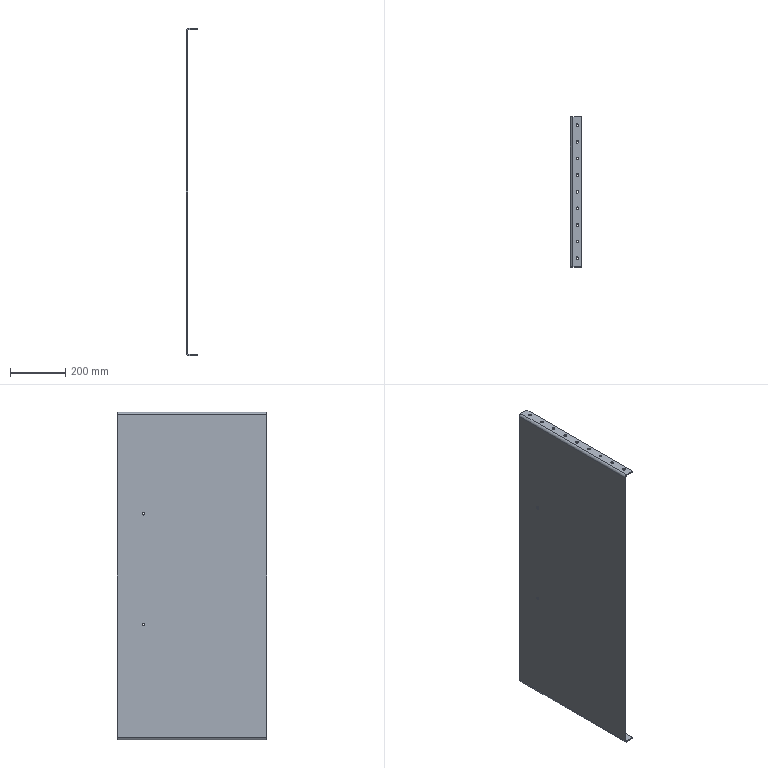Part | SolidWorks | features HoleWzd 3, LPattern 2, EdgeFlange 1, FlatPattern 1, MirrorPattern 1, SMBaseFlange 1, SheetMetal 1, UnFold 1, WeldmentFeature 1 | 1 solid | 62 faces | box 40 x 540 x 1180 mm | volume 2685058 mm3 | cylinder 44 | plane 18 | commonest cylinder face diameters 10 x42 18 x2